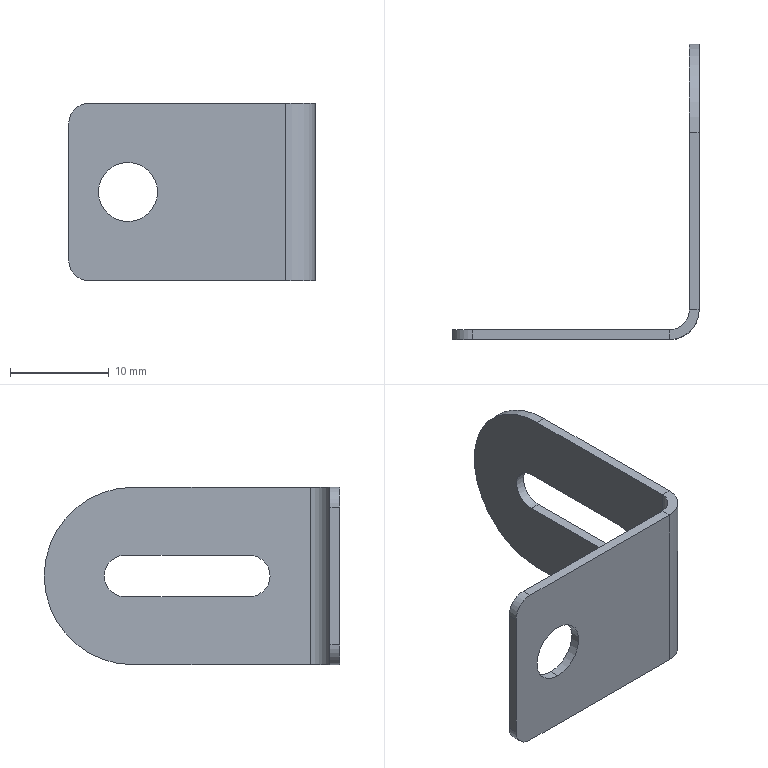Part | SolidWorks | features Fillet 2, ICE 2, EdgeFlange 1, FlatPattern 1, SMBaseFlange 1, SheetMetal 1 | 1 solid | 24 faces | box 25 x 30 x 18 mm | volume 820.964 mm3 | plane 13 | cylinder 11 | commonest cylinder face diameters 4 x3 4.2 x3 6 x3 18 x2
STEP:
#1=CARTESIAN_POINT('',(12.5,8.173,2.1));
#2=VERTEX_POINT('',#1);
#3=CARTESIAN_POINT('',(12.5,6.073,0.));
#4=VERTEX_POINT('',#3);
#5=CARTESIAN_POINT('',(12.5,8.173,0.));
#6=DIRECTION('',(1.,0.,0.));
#7=DIRECTION('',(0.,1.,0.));
#8=AXIS2_PLACEMENT_3D('',#5,#6,#7);
#9=CIRCLE('',#8,2.1);
#10=EDGE_CURVE('',#2,#4,#9,.T.);
#11=ORIENTED_EDGE('',*,*,#10,.T.);
#12=CARTESIAN_POINT('',(11.5,6.073,0.));
#13=VERTEX_POINT('',#12);
#14=CARTESIAN_POINT('',(21.5,6.073,0.));
#15=DIRECTION('',(-1.,0.,0.));
#16=VECTOR('',#15,1000.);
#17=LINE('',#14,#16);
#18=EDGE_CURVE('',#4,#13,#17,.T.);
#19=ORIENTED_EDGE('',*,*,#18,.T.);
#20=CARTESIAN_POINT('',(11.5,8.173,2.1));
#21=VERTEX_POINT('',#20);
#22=CARTESIAN_POINT('',(11.5,8.173,0.));
#23=DIRECTION('',(-1.,0.,0.));
#24=DIRECTION('',(0.,-1.,0.));
#25=AXIS2_PLACEMENT_3D('',#22,#23,#24);
#26=CIRCLE('',#25,2.1);
#27=EDGE_CURVE('',#13,#21,#26,.T.);
#28=ORIENTED_EDGE('',*,*,#27,.T.);
#29=CARTESIAN_POINT('',(21.5,8.173,2.1));
#30=DIRECTION('',(-1.,0.,0.));
#31=VECTOR('',#30,1000.);
#32=LINE('',#29,#31);
#33=EDGE_CURVE('',#2,#21,#32,.T.);
#34=ORIENTED_EDGE('',*,*,#33,.F.);
#35=EDGE_LOOP('',(#11,#19,#28,#34));
#36=FACE_OUTER_BOUND('',#35,.T.);
#37=CARTESIAN_POINT('',(21.5,8.173,0.));
#38=DIRECTION('',(-1.,0.,0.));
#39=DIRECTION('',(0.,-1.,0.));
#40=AXIS2_PLACEMENT_3D('',#37,#38,#39);
#41=CYLINDRICAL_SURFACE('',#40,2.1);
#42=ADVANCED_FACE('',(#36),#41,.F.);
#43=CARTESIAN_POINT('',(-6.5,-1.,-3.));
#44=VERTEX_POINT('',#43);
#45=CARTESIAN_POINT('',(-6.5,-1.,3.));
#46=VERTEX_POINT('',#45);
#47=CARTESIAN_POINT('',(-6.5,-1.,0.));
#48=DIRECTION('',(0.,1.,0.));
#49=DIRECTION('',(0.,0.,1.));
#50=AXIS2_PLACEMENT_3D('',#47,#48,#49);
#51=CIRCLE('',#50,3.);
#52=EDGE_CURVE('',#44,#46,#51,.T.);
#53=ORIENTED_EDGE('',*,*,#52,.F.);
#54=CARTESIAN_POINT('',(-6.5,0.,-3.));
#55=VERTEX_POINT('',#54);
#56=CARTESIAN_POINT('',(-6.5,-10.,-3.));
#57=DIRECTION('',(0.,1.,0.));
#58=VECTOR('',#57,1000.);
#59=LINE('',#56,#58);
#60=EDGE_CURVE('',#44,#55,#59,.T.);
#61=ORIENTED_EDGE('',*,*,#60,.T.);
#62=CARTESIAN_POINT('',(-6.5,0.,3.));
#63=VERTEX_POINT('',#62);
#64=CARTESIAN_POINT('',(-6.5,0.,0.));
#65=DIRECTION('',(0.,1.,0.));
#66=DIRECTION('',(0.,0.,1.));
#67=AXIS2_PLACEMENT_3D('',#64,#65,#66);
#68=CIRCLE('',#67,3.);
#69=EDGE_CURVE('',#55,#63,#68,.T.);
#70=ORIENTED_EDGE('',*,*,#69,.T.);
#71=CARTESIAN_POINT('',(-6.5,-10.,3.));
#72=DIRECTION('',(0.,1.,0.));
#73=VECTOR('',#72,1000.);
#74=LINE('',#71,#73);
#75=EDGE_CURVE('',#46,#63,#74,.T.);
#76=ORIENTED_EDGE('',*,*,#75,.F.);
#77=EDGE_LOOP('',(#53,#61,#70,#76));
#78=FACE_OUTER_BOUND('',#77,.T.);
#79=CARTESIAN_POINT('',(-6.5,-10.,0.));
#80=DIRECTION('',(0.,1.,0.));
#81=DIRECTION('',(0.,0.,1.));
#82=AXIS2_PLACEMENT_3D('',#79,#80,#81);
#83=CYLINDRICAL_SURFACE('',#82,3.);
#84=ADVANCED_FACE('',(#78),#83,.F.);
#85=CARTESIAN_POINT('',(9.5,-1.,-9.));
#86=VERTEX_POINT('',#85);
#87=CARTESIAN_POINT('',(-10.5,-1.,-9.));
#88=VERTEX_POINT('',#87);
#89=CARTESIAN_POINT('',(-12.5,-1.,-9.));
#90=DIRECTION('',(-1.,0.,0.));
#91=VECTOR('',#90,1000.);
#92=LINE('',#89,#91);
#93=EDGE_CURVE('',#86,#88,#92,.T.);
#94=ORIENTED_EDGE('',*,*,#93,.T.);
#95=CARTESIAN_POINT('',(-10.5,0.,-9.));
#96=VERTEX_POINT('',#95);
#97=CARTESIAN_POINT('',(-10.5,-1.,-9.));
#98=DIRECTION('',(0.,1.,0.));
#99=VECTOR('',#98,1000.);
#100=LINE('',#97,#99);
#101=EDGE_CURVE('',#88,#96,#100,.T.);
#102=ORIENTED_EDGE('',*,*,#101,.T.);
#103=CARTESIAN_POINT('',(9.5,0.,-9.));
#104=VERTEX_POINT('',#103);
#105=CARTESIAN_POINT('',(-12.5,0.,-9.));
#106=DIRECTION('',(-1.,0.,0.));
#107=VECTOR('',#106,1000.);
#108=LINE('',#105,#107);
#109=EDGE_CURVE('',#104,#96,#108,.T.);
#110=ORIENTED_EDGE('',*,*,#109,.F.);
#111=CARTESIAN_POINT('',(9.5,0.,-9.));
#112=DIRECTION('',(0.,-1.,0.));
#113=VECTOR('',#112,1000.);
#114=LINE('',#111,#113);
#115=EDGE_CURVE('',#104,#86,#114,.T.);
#116=ORIENTED_EDGE('',*,*,#115,.T.);
#117=EDGE_LOOP('',(#94,#102,#110,#116));
#118=FACE_OUTER_BOUND('',#117,.T.);
#119=CARTESIAN_POINT('',(-12.5,-1.,-9.));
#120=DIRECTION('',(0.,0.,-1.));
#121=DIRECTION('',(-1.,0.,0.));
#122=AXIS2_PLACEMENT_3D('',#119,#120,#121);
#123=PLANE('',#122);
#124=ADVANCED_FACE('',(#118),#123,.T.);
#125=CARTESIAN_POINT('',(-6.5,-1.,0.));
#126=DIRECTION('',(0.,1.,0.));
#127=DIRECTION('',(0.,0.,1.));
#128=AXIS2_PLACEMENT_3D('',#125,#126,#127);
#129=CIRCLE('',#128,3.);
#130=EDGE_CURVE('',#46,#44,#129,.T.);
#131=ORIENTED_EDGE('',*,*,#130,.T.);
#132=ORIENTED_EDGE('',*,*,#52,.T.);
#133=EDGE_LOOP('',(#131,#132));
#134=FACE_BOUND('',#133,.T.);
#135=CARTESIAN_POINT('',(-12.5,-1.,-7.));
#136=VERTEX_POINT('',#135);
#137=CARTESIAN_POINT('',(-12.5,-1.,7.));
#138=VERTEX_POINT('',#137);
#139=CARTESIAN_POINT('',(-12.5,-1.,-9.));
#140=DIRECTION('',(0.,0.,1.));
#141=VECTOR('',#140,1000.);
#142=LINE('',#139,#141);
#143=EDGE_CURVE('',#136,#138,#142,.T.);
#144=ORIENTED_EDGE('',*,*,#143,.F.);
#145=CARTESIAN_POINT('',(-10.5,-1.,-7.));
#146=DIRECTION('',(0.,-1.,0.));
#147=DIRECTION('',(0.,0.,1.));
#148=AXIS2_PLACEMENT_3D('',#145,#146,#147);
#149=CIRCLE('',#148,2.);
#150=EDGE_CURVE('',#136,#88,#149,.T.);
#151=ORIENTED_EDGE('',*,*,#150,.T.);
#152=ORIENTED_EDGE('',*,*,#93,.F.);
#153=CARTESIAN_POINT('',(9.5,-1.,9.));
#154=VERTEX_POINT('',#153);
#155=CARTESIAN_POINT('',(9.5,-1.,-9.));
#156=DIRECTION('',(0.,0.,1.));
#157=VECTOR('',#156,1000.);
#158=LINE('',#155,#157);
#159=EDGE_CURVE('',#86,#154,#158,.T.);
#160=ORIENTED_EDGE('',*,*,#159,.T.);
#161=CARTESIAN_POINT('',(-10.5,-1.,9.));
#162=VERTEX_POINT('',#161);
#163=CARTESIAN_POINT('',(-12.5,-1.,9.));
#164=DIRECTION('',(1.,0.,0.));
#165=VECTOR('',#164,1000.);
#166=LINE('',#163,#165);
#167=EDGE_CURVE('',#162,#154,#166,.T.);
#168=ORIENTED_EDGE('',*,*,#167,.F.);
#169=CARTESIAN_POINT('',(-10.5,-1.,7.));
#170=DIRECTION('',(0.,-1.,0.));
#171=DIRECTION('',(0.,0.,1.));
#172=AXIS2_PLACEMENT_3D('',#169,#170,#171);
#173=CIRCLE('',#172,2.);
#174=EDGE_CURVE('',#162,#138,#173,.T.);
#175=ORIENTED_EDGE('',*,*,#174,.T.);
#176=EDGE_LOOP('',(#144,#151,#152,#160,#168,#175));
#177=FACE_OUTER_BOUND('',#176,.T.);
#178=CARTESIAN_POINT('',(0.,-1.,0.));
#179=DIRECTION('',(0.,1.,0.));
#180=DIRECTION('',(0.,0.,1.));
#181=AXIS2_PLACEMENT_3D('',#178,#179,#180);
#182=PLANE('',#181);
#183=ADVANCED_FACE('',(#134,#177),#182,.F.);
#184=CARTESIAN_POINT('',(-6.5,0.,0.));
#185=DIRECTION('',(0.,1.,0.));
#186=DIRECTION('',(0.,0.,1.));
#187=AXIS2_PLACEMENT_3D('',#184,#185,#186);
#188=CIRCLE('',#187,3.);
#189=EDGE_CURVE('',#63,#55,#188,.T.);
#190=ORIENTED_EDGE('',*,*,#189,.F.);
#191=ORIENTED_EDGE('',*,*,#69,.F.);
#192=EDGE_LOOP('',(#190,#191));
#193=FACE_BOUND('',#192,.T.);
#194=ORIENTED_EDGE('',*,*,#109,.T.);
#195=CARTESIAN_POINT('',(-12.5,0.,-7.));
#196=VERTEX_POINT('',#195);
#197=CARTESIAN_POINT('',(-10.5,0.,-7.));
#198=DIRECTION('',(0.,1.,0.));
#199=DIRECTION('',(0.,0.,1.));
#200=AXIS2_PLACEMENT_3D('',#197,#198,#199);
#201=CIRCLE('',#200,2.);
#202=EDGE_CURVE('',#96,#196,#201,.T.);
#203=ORIENTED_EDGE('',*,*,#202,.T.);
#204=CARTESIAN_POINT('',(-12.5,0.,7.));
#205=VERTEX_POINT('',#204);
#206=CARTESIAN_POINT('',(-12.5,0.,-9.));
#207=DIRECTION('',(0.,0.,1.));
#208=VECTOR('',#207,1000.);
#209=LINE('',#206,#208);
#210=EDGE_CURVE('',#196,#205,#209,.T.);
#211=ORIENTED_EDGE('',*,*,#210,.T.);
#212=CARTESIAN_POINT('',(-10.5,0.,9.));
#213=VERTEX_POINT('',#212);
#214=CARTESIAN_POINT('',(-10.5,0.,7.));
#215=DIRECTION('',(0.,1.,0.));
#216=DIRECTION('',(0.,0.,1.));
#217=AXIS2_PLACEMENT_3D('',#214,#215,#216);
#218=CIRCLE('',#217,2.);
#219=EDGE_CURVE('',#205,#213,#218,.T.);
#220=ORIENTED_EDGE('',*,*,#219,.T.);
#221=CARTESIAN_POINT('',(9.5,0.,9.));
#222=VERTEX_POINT('',#221);
#223=CARTESIAN_POINT('',(-12.5,0.,9.));
#224=DIRECTION('',(1.,0.,0.));
#225=VECTOR('',#224,1000.);
#226=LINE('',#223,#225);
#227=EDGE_CURVE('',#213,#222,#226,.T.);
#228=ORIENTED_EDGE('',*,*,#227,.T.);
#229=CARTESIAN_POINT('',(9.5,0.,-9.));
#230=DIRECTION('',(0.,0.,1.));
#231=VECTOR('',#230,1000.);
#232=LINE('',#229,#231);
#233=EDGE_CURVE('',#104,#222,#232,.T.);
#234=ORIENTED_EDGE('',*,*,#233,.F.);
#235=EDGE_LOOP('',(#194,#203,#211,#220,#228,#234));
#236=FACE_OUTER_BOUND('',#235,.T.);
#237=CARTESIAN_POINT('',(0.,0.,0.));
#238=DIRECTION('',(0.,1.,0.));
#239=DIRECTION('',(0.,0.,1.));
#240=AXIS2_PLACEMENT_3D('',#237,#238,#239);
#241=PLANE('',#240);
#242=ADVANCED_FACE('',(#193,#236),#241,.T.);
#243=ORIENTED_EDGE('',*,*,#227,.F.);
#244=CARTESIAN_POINT('',(-10.5,-1.,9.));
#245=DIRECTION('',(0.,-1.,0.));
#246=VECTOR('',#245,1000.);
#247=LINE('',#244,#246);
#248=EDGE_CURVE('',#213,#162,#247,.T.);
#249=ORIENTED_EDGE('',*,*,#248,.T.);
#250=ORIENTED_EDGE('',*,*,#167,.T.);
#251=CARTESIAN_POINT('',(9.5,0.,9.));
#252=DIRECTION('',(0.,-1.,0.));
#253=VECTOR('',#252,1000.);
#254=LINE('',#251,#253);
#255=EDGE_CURVE('',#222,#154,#254,.T.);
#256=ORIENTED_EDGE('',*,*,#255,.F.);
#257=EDGE_LOOP('',(#243,#249,#250,#256));
#258=FACE_OUTER_BOUND('',#257,.T.);
#259=CARTESIAN_POINT('',(-12.5,-1.,9.));
#260=DIRECTION('',(0.,0.,1.));
#261=DIRECTION('',(1.,0.,0.));
#262=AXIS2_PLACEMENT_3D('',#259,#260,#261);
#263=PLANE('',#262);
#264=ADVANCED_FACE('',(#258),#263,.T.);
#265=ORIENTED_EDGE('',*,*,#210,.F.);
#266=CARTESIAN_POINT('',(-12.5,-1.,-7.));
#267=DIRECTION('',(0.,-1.,0.));
#268=VECTOR('',#267,1000.);
#269=LINE('',#266,#268);
#270=EDGE_CURVE('',#196,#136,#269,.T.);
#271=ORIENTED_EDGE('',*,*,#270,.T.);
#272=ORIENTED_EDGE('',*,*,#143,.T.);
#273=CARTESIAN_POINT('',(-12.5,-1.,7.));
#274=DIRECTION('',(0.,1.,0.));
#275=VECTOR('',#274,1000.);
#276=LINE('',#273,#275);
#277=EDGE_CURVE('',#138,#205,#276,.T.);
#278=ORIENTED_EDGE('',*,*,#277,.T.);
#279=EDGE_LOOP('',(#265,#271,#272,#278));
#280=FACE_OUTER_BOUND('',#279,.T.);
#281=CARTESIAN_POINT('',(-12.5,-1.,-9.));
#282=DIRECTION('',(-1.,0.,0.));
#283=DIRECTION('',(0.,0.,1.));
#284=AXIS2_PLACEMENT_3D('',#281,#282,#283);
#285=PLANE('',#284);
#286=ADVANCED_FACE('',(#280),#285,.T.);
#287=CARTESIAN_POINT('',(11.5,2.,9.));
#288=VERTEX_POINT('',#287);
#289=CARTESIAN_POINT('',(12.5,2.,9.));
#290=VERTEX_POINT('',#289);
#291=CARTESIAN_POINT('',(12.5,2.,9.));
#292=DIRECTION('',(1.,0.,0.));
#293=VECTOR('',#292,1000.);
#294=LINE('',#291,#293);
#295=EDGE_CURVE('',#288,#290,#294,.T.);
#296=ORIENTED_EDGE('',*,*,#295,.F.);
#297=CARTESIAN_POINT('',(9.5,2.,9.));
#298=DIRECTION('',(0.,0.,1.));
#299=DIRECTION('',(-1.,0.,0.));
#300=AXIS2_PLACEMENT_3D('',#297,#298,#299);
#301=CIRCLE('',#300,2.);
#302=EDGE_CURVE('',#222,#288,#301,.T.);
#303=ORIENTED_EDGE('',*,*,#302,.F.);
#304=ORIENTED_EDGE('',*,*,#255,.T.);
#305=CARTESIAN_POINT('',(9.5,2.,9.));
#306=DIRECTION('',(0.,0.,1.));
#307=DIRECTION('',(-1.,0.,0.));
#308=AXIS2_PLACEMENT_3D('',#305,#306,#307);
#309=CIRCLE('',#308,3.);
#310=EDGE_CURVE('',#154,#290,#309,.T.);
#311=ORIENTED_EDGE('',*,*,#310,.T.);
#312=EDGE_LOOP('',(#296,#303,#304,#311));
#313=FACE_OUTER_BOUND('',#312,.T.);
#314=CARTESIAN_POINT('',(9.5,2.,9.));
#315=DIRECTION('',(0.,0.,1.));
#316=DIRECTION('',(1.,0.,0.));
#317=AXIS2_PLACEMENT_3D('',#314,#315,#316);
#318=PLANE('',#317);
#319=ADVANCED_FACE('',(#313),#318,.T.);
#320=CARTESIAN_POINT('',(11.5,2.,-9.));
#321=VERTEX_POINT('',#320);
#322=CARTESIAN_POINT('',(9.5,2.,-9.));
#323=DIRECTION('',(0.,0.,-1.));
#324=DIRECTION('',(-1.,0.,0.));
#325=AXIS2_PLACEMENT_3D('',#322,#323,#324);
#326=CIRCLE('',#325,2.);
#327=EDGE_CURVE('',#321,#104,#326,.T.);
#328=ORIENTED_EDGE('',*,*,#327,.F.);
#329=CARTESIAN_POINT('',(12.5,2.,-9.));
#330=VERTEX_POINT('',#329);
#331=CARTESIAN_POINT('',(11.5,2.,-9.));
#332=DIRECTION('',(1.,0.,0.));
#333=VECTOR('',#332,1000.);
#334=LINE('',#331,#333);
#335=EDGE_CURVE('',#321,#330,#334,.T.);
#336=ORIENTED_EDGE('',*,*,#335,.T.);
#337=CARTESIAN_POINT('',(9.5,2.,-9.));
#338=DIRECTION('',(0.,0.,-1.));
#339=DIRECTION('',(-1.,0.,0.));
#340=AXIS2_PLACEMENT_3D('',#337,#338,#339);
#341=CIRCLE('',#340,3.);
#342=EDGE_CURVE('',#330,#86,#341,.T.);
#343=ORIENTED_EDGE('',*,*,#342,.T.);
#344=ORIENTED_EDGE('',*,*,#115,.F.);
#345=EDGE_LOOP('',(#328,#336,#343,#344));
#346=FACE_OUTER_BOUND('',#345,.T.);
#347=CARTESIAN_POINT('',(9.5,2.,-9.));
#348=DIRECTION('',(0.,0.,1.));
#349=DIRECTION('',(1.,0.,0.));
#350=AXIS2_PLACEMENT_3D('',#347,#348,#349);
#351=PLANE('',#350);
#352=ADVANCED_FACE('',(#346),#351,.F.);
#353=ORIENTED_EDGE('',*,*,#159,.F.);
#354=ORIENTED_EDGE('',*,*,#342,.F.);
#355=CARTESIAN_POINT('',(12.5,2.,0.));
#356=DIRECTION('',(0.,0.,-1.));
#357=VECTOR('',#356,1000.);
#358=LINE('',#355,#357);
#359=EDGE_CURVE('',#290,#330,#358,.T.);
#360=ORIENTED_EDGE('',*,*,#359,.F.);
#361=ORIENTED_EDGE('',*,*,#310,.F.);
#362=EDGE_LOOP('',(#353,#354,#360,#361));
#363=FACE_OUTER_BOUND('',#362,.T.);
#364=CARTESIAN_POINT('',(9.5,2.,-9.));
#365=DIRECTION('',(0.,0.,-1.));
#366=DIRECTION('',(1.,0.,0.));
#367=AXIS2_PLACEMENT_3D('',#364,#365,#366);
#368=CYLINDRICAL_SURFACE('',#367,3.);
#369=ADVANCED_FACE('',(#363),#368,.T.);
#370=ORIENTED_EDGE('',*,*,#233,.T.);
#371=ORIENTED_EDGE('',*,*,#302,.T.);
#372=CARTESIAN_POINT('',(11.5,2.,9.));
#373=DIRECTION('',(0.,0.,-1.));
#374=VECTOR('',#373,1000.);
#375=LINE('',#372,#374);
#376=EDGE_CURVE('',#288,#321,#375,.T.);
#377=ORIENTED_EDGE('',*,*,#376,.T.);
#378=ORIENTED_EDGE('',*,*,#327,.T.);
#379=EDGE_LOOP('',(#370,#371,#377,#378));
#380=FACE_OUTER_BOUND('',#379,.T.);
#381=CARTESIAN_POINT('',(9.5,2.,-9.));
#382=DIRECTION('',(0.,0.,-1.));
#383=DIRECTION('',(1.,0.,0.));
#384=AXIS2_PLACEMENT_3D('',#381,#382,#383);
#385=CYLINDRICAL_SURFACE('',#384,2.);
#386=ADVANCED_FACE('',(#380),#385,.F.);
#387=CARTESIAN_POINT('',(11.5,20.,-9.));
#388=VERTEX_POINT('',#387);
#389=CARTESIAN_POINT('',(11.5,0.,-9.));
#390=DIRECTION('',(0.,-1.,0.));
#391=VECTOR('',#390,1000.);
#392=LINE('',#389,#391);
#393=EDGE_CURVE('',#388,#321,#392,.T.);
#394=ORIENTED_EDGE('',*,*,#393,.F.);
#395=CARTESIAN_POINT('',(12.5,20.,-9.));
#396=VERTEX_POINT('',#395);
#397=CARTESIAN_POINT('',(12.5,20.,-9.));
#398=DIRECTION('',(1.,0.,0.));
#399=VECTOR('',#398,1000.);
#400=LINE('',#397,#399);
#401=EDGE_CURVE('',#388,#396,#400,.T.);
#402=ORIENTED_EDGE('',*,*,#401,.T.);
#403=CARTESIAN_POINT('',(12.5,0.,-9.));
#404=DIRECTION('',(0.,-1.,0.));
#405=VECTOR('',#404,1000.);
#406=LINE('',#403,#405);
#407=EDGE_CURVE('',#396,#330,#406,.T.);
#408=ORIENTED_EDGE('',*,*,#407,.T.);
#409=ORIENTED_EDGE('',*,*,#335,.F.);
#410=EDGE_LOOP('',(#394,#402,#408,#409));
#411=FACE_OUTER_BOUND('',#410,.T.);
#412=CARTESIAN_POINT('',(12.5,0.,-9.));
#413=DIRECTION('',(0.,0.,-1.));
#414=DIRECTION('',(-1.,0.,0.));
#415=AXIS2_PLACEMENT_3D('',#412,#413,#414);
#416=PLANE('',#415);
#417=ADVANCED_FACE('',(#411),#416,.T.);
#418=CARTESIAN_POINT('',(12.5,20.,9.));
#419=VERTEX_POINT('',#418);
#420=CARTESIAN_POINT('',(12.5,29.,9.));
#421=DIRECTION('',(0.,1.,0.));
#422=VECTOR('',#421,1000.);
#423=LINE('',#420,#422);
#424=EDGE_CURVE('',#290,#419,#423,.T.);
#425=ORIENTED_EDGE('',*,*,#424,.T.);
#426=CARTESIAN_POINT('',(11.5,20.,9.));
#427=VERTEX_POINT('',#426);
#428=CARTESIAN_POINT('',(12.5,20.,9.));
#429=DIRECTION('',(-1.,0.,0.));
#430=VECTOR('',#429,1000.);
#431=LINE('',#428,#430);
#432=EDGE_CURVE('',#419,#427,#431,.T.);
#433=ORIENTED_EDGE('',*,*,#432,.T.);
#434=CARTESIAN_POINT('',(11.5,0.,9.));
#435=DIRECTION('',(0.,1.,0.));
#436=VECTOR('',#435,1000.);
#437=LINE('',#434,#436);
#438=EDGE_CURVE('',#288,#427,#437,.T.);
#439=ORIENTED_EDGE('',*,*,#438,.F.);
#440=ORIENTED_EDGE('',*,*,#295,.T.);
#441=EDGE_LOOP('',(#425,#433,#439,#440));
#442=FACE_OUTER_BOUND('',#441,.T.);
#443=CARTESIAN_POINT('',(12.5,29.,9.));
#444=DIRECTION('',(0.,0.,1.));
#445=DIRECTION('',(1.,0.,0.));
#446=AXIS2_PLACEMENT_3D('',#443,#444,#445);
#447=PLANE('',#446);
#448=ADVANCED_FACE('',(#442),#447,.T.);
#449=CARTESIAN_POINT('',(12.5,20.819,-2.1));
#450=VERTEX_POINT('',#449);
#451=CARTESIAN_POINT('',(12.5,20.819,2.1));
#452=VERTEX_POINT('',#451);
#453=CARTESIAN_POINT('',(12.5,20.819,0.));
#454=DIRECTION('',(1.,0.,0.));
#455=DIRECTION('',(0.,1.,0.));
#456=AXIS2_PLACEMENT_3D('',#453,#454,#455);
#457=CIRCLE('',#456,2.1);
#458=EDGE_CURVE('',#450,#452,#457,.T.);
#459=ORIENTED_EDGE('',*,*,#458,.F.);
#460=CARTESIAN_POINT('',(12.5,8.173,-2.1));
#461=VERTEX_POINT('',#460);
#462=CARTESIAN_POINT('',(12.5,0.,-2.1));
#463=DIRECTION('',(0.,1.,0.));
#464=VECTOR('',#463,1000.);
#465=LINE('',#462,#464);
#466=EDGE_CURVE('',#461,#450,#465,.T.);
#467=ORIENTED_EDGE('',*,*,#466,.F.);
#468=CARTESIAN_POINT('',(12.5,8.173,0.));
#469=DIRECTION('',(1.,0.,0.));
#470=DIRECTION('',(0.,1.,0.));
#471=AXIS2_PLACEMENT_3D('',#468,#469,#470);
#472=CIRCLE('',#471,2.1);
#473=EDGE_CURVE('',#4,#461,#472,.T.);
#474=ORIENTED_EDGE('',*,*,#473,.F.);
#475=ORIENTED_EDGE('',*,*,#10,.F.);
#476=CARTESIAN_POINT('',(12.5,0.,2.1));
#477=DIRECTION('',(0.,-1.,0.));
#478=VECTOR('',#477,1000.);
#479=LINE('',#476,#478);
#480=EDGE_CURVE('',#452,#2,#479,.T.);
#481=ORIENTED_EDGE('',*,*,#480,.F.);
#482=EDGE_LOOP('',(#459,#467,#474,#475,#481));
#483=FACE_BOUND('',#482,.T.);
#484=ORIENTED_EDGE('',*,*,#407,.F.);
#485=CARTESIAN_POINT('',(12.5,29.,0.));
#486=VERTEX_POINT('',#485);
#487=CARTESIAN_POINT('',(12.5,20.,0.));
#488=DIRECTION('',(1.,0.,0.));
#489=DIRECTION('',(0.,1.,0.));
#490=AXIS2_PLACEMENT_3D('',#487,#488,#489);
#491=CIRCLE('',#490,9.);
#492=EDGE_CURVE('',#396,#486,#491,.T.);
#493=ORIENTED_EDGE('',*,*,#492,.T.);
#494=CARTESIAN_POINT('',(12.5,20.,0.));
#495=DIRECTION('',(1.,0.,0.));
#496=DIRECTION('',(0.,1.,0.));
#497=AXIS2_PLACEMENT_3D('',#494,#495,#496);
#498=CIRCLE('',#497,9.);
#499=EDGE_CURVE('',#486,#419,#498,.T.);
#500=ORIENTED_EDGE('',*,*,#499,.T.);
#501=ORIENTED_EDGE('',*,*,#424,.F.);
#502=ORIENTED_EDGE('',*,*,#359,.T.);
#503=EDGE_LOOP('',(#484,#493,#500,#501,#502));
#504=FACE_OUTER_BOUND('',#503,.T.);
#505=CARTESIAN_POINT('',(12.5,0.,0.));
#506=DIRECTION('',(1.,0.,0.));
#507=DIRECTION('',(0.,1.,0.));
#508=AXIS2_PLACEMENT_3D('',#505,#506,#507);
#509=PLANE('',#508);
#510=ADVANCED_FACE('',(#483,#504),#509,.T.);
#511=CARTESIAN_POINT('',(11.5,20.819,-2.1));
#512=VERTEX_POINT('',#511);
#513=CARTESIAN_POINT('',(11.5,8.173,-2.1));
#514=VERTEX_POINT('',#513);
#515=CARTESIAN_POINT('',(11.5,20.819,-2.1));
#516=DIRECTION('',(0.,-1.,0.));
#517=VECTOR('',#516,1000.);
#518=LINE('',#515,#517);
#519=EDGE_CURVE('',#512,#514,#518,.T.);
#520=ORIENTED_EDGE('',*,*,#519,.F.);
#521=CARTESIAN_POINT('',(11.5,20.819,2.1));
#522=VERTEX_POINT('',#521);
#523=CARTESIAN_POINT('',(11.5,20.819,0.));
#524=DIRECTION('',(-1.,0.,0.));
#525=DIRECTION('',(0.,-1.,0.));
#526=AXIS2_PLACEMENT_3D('',#523,#524,#525);
#527=CIRCLE('',#526,2.1);
#528=EDGE_CURVE('',#522,#512,#527,.T.);
#529=ORIENTED_EDGE('',*,*,#528,.F.);
#530=CARTESIAN_POINT('',(11.5,20.819,2.1));
#531=DIRECTION('',(0.,1.,0.));
#532=VECTOR('',#531,1000.);
#533=LINE('',#530,#532);
#534=EDGE_CURVE('',#21,#522,#533,.T.);
#535=ORIENTED_EDGE('',*,*,#534,.F.);
#536=ORIENTED_EDGE('',*,*,#27,.F.);
#537=CARTESIAN_POINT('',(11.5,8.173,0.));
#538=DIRECTION('',(-1.,0.,0.));
#539=DIRECTION('',(0.,-1.,0.));
#540=AXIS2_PLACEMENT_3D('',#537,#538,#539);
#541=CIRCLE('',#540,2.1);
#542=EDGE_CURVE('',#514,#13,#541,.T.);
#543=ORIENTED_EDGE('',*,*,#542,.F.);
#544=EDGE_LOOP('',(#520,#529,#535,#536,#543));
#545=FACE_BOUND('',#544,.T.);
#546=CARTESIAN_POINT('',(11.5,29.,0.));
#547=VERTEX_POINT('',#546);
#548=CARTESIAN_POINT('',(11.5,20.,0.));
#549=DIRECTION('',(-1.,0.,0.));
#550=DIRECTION('',(0.,1.,0.));
#551=AXIS2_PLACEMENT_3D('',#548,#549,#550);
#552=CIRCLE('',#551,9.);
#553=EDGE_CURVE('',#427,#547,#552,.T.);
#554=ORIENTED_EDGE('',*,*,#553,.T.);
#555=CARTESIAN_POINT('',(11.5,20.,0.));
#556=DIRECTION('',(-1.,0.,0.));
#557=DIRECTION('',(0.,1.,0.));
#558=AXIS2_PLACEMENT_3D('',#555,#556,#557);
#559=CIRCLE('',#558,9.);
#560=EDGE_CURVE('',#547,#388,#559,.T.);
#561=ORIENTED_EDGE('',*,*,#560,.T.);
#562=ORIENTED_EDGE('',*,*,#393,.T.);
#563=ORIENTED_EDGE('',*,*,#376,.F.);
#564=ORIENTED_EDGE('',*,*,#438,.T.);
#565=EDGE_LOOP('',(#554,#561,#562,#563,#564));
#566=FACE_OUTER_BOUND('',#565,.T.);
#567=CARTESIAN_POINT('',(11.5,0.,0.));
#568=DIRECTION('',(1.,0.,0.));
#569=DIRECTION('',(0.,1.,0.));
#570=AXIS2_PLACEMENT_3D('',#567,#568,#569);
#571=PLANE('',#570);
#572=ADVANCED_FACE('',(#545,#566),#571,.F.);
#573=ORIENTED_EDGE('',*,*,#60,.F.);
#574=ORIENTED_EDGE('',*,*,#130,.F.);
#575=ORIENTED_EDGE('',*,*,#75,.T.);
#576=ORIENTED_EDGE('',*,*,#189,.T.);
#577=EDGE_LOOP('',(#573,#574,#575,#576));
#578=FACE_OUTER_BOUND('',#577,.T.);
#579=CARTESIAN_POINT('',(-6.5,-10.,0.));
#580=DIRECTION('',(0.,1.,0.));
#581=DIRECTION('',(0.,0.,1.));
#582=AXIS2_PLACEMENT_3D('',#579,#580,#581);
#583=CYLINDRICAL_SURFACE('',#582,3.);
#584=ADVANCED_FACE('',(#578),#583,.F.);
#585=ORIENTED_EDGE('',*,*,#432,.F.);
#586=ORIENTED_EDGE('',*,*,#499,.F.);
#587=CARTESIAN_POINT('',(12.5,29.,0.));
#588=DIRECTION('',(1.,0.,0.));
#589=VECTOR('',#588,1000.);
#590=LINE('',#587,#589);
#591=EDGE_CURVE('',#547,#486,#590,.T.);
#592=ORIENTED_EDGE('',*,*,#591,.F.);
#593=ORIENTED_EDGE('',*,*,#553,.F.);
#594=EDGE_LOOP('',(#585,#586,#592,#593));
#595=FACE_OUTER_BOUND('',#594,.T.);
#596=CARTESIAN_POINT('',(12.5,20.,0.));
#597=DIRECTION('',(-1.,0.,0.));
#598=DIRECTION('',(0.,-1.,0.));
#599=AXIS2_PLACEMENT_3D('',#596,#597,#598);
#600=CYLINDRICAL_SURFACE('',#599,9.);
#601=ADVANCED_FACE('',(#595),#600,.T.);
#602=ORIENTED_EDGE('',*,*,#492,.F.);
#603=ORIENTED_EDGE('',*,*,#401,.F.);
#604=ORIENTED_EDGE('',*,*,#560,.F.);
#605=ORIENTED_EDGE('',*,*,#591,.T.);
#606=EDGE_LOOP('',(#602,#603,#604,#605));
#607=FACE_OUTER_BOUND('',#606,.T.);
#608=CARTESIAN_POINT('',(12.5,20.,0.));
#609=DIRECTION('',(-1.,0.,0.));
#610=DIRECTION('',(0.,-1.,0.));
#611=AXIS2_PLACEMENT_3D('',#608,#609,#610);
#612=CYLINDRICAL_SURFACE('',#611,9.);
#613=ADVANCED_FACE('',(#607),#612,.T.);
#614=ORIENTED_EDGE('',*,*,#458,.T.);
#615=CARTESIAN_POINT('',(21.5,20.819,2.1));
#616=DIRECTION('',(-1.,0.,0.));
#617=VECTOR('',#616,1000.);
#618=LINE('',#615,#617);
#619=EDGE_CURVE('',#452,#522,#618,.T.);
#620=ORIENTED_EDGE('',*,*,#619,.T.);
#621=ORIENTED_EDGE('',*,*,#528,.T.);
#622=CARTESIAN_POINT('',(21.5,20.819,-2.1));
#623=DIRECTION('',(-1.,0.,0.));
#624=VECTOR('',#623,1000.);
#625=LINE('',#622,#624);
#626=EDGE_CURVE('',#450,#512,#625,.T.);
#627=ORIENTED_EDGE('',*,*,#626,.F.);
#628=EDGE_LOOP('',(#614,#620,#621,#627));
#629=FACE_OUTER_BOUND('',#628,.T.);
#630=CARTESIAN_POINT('',(21.5,20.819,0.));
#631=DIRECTION('',(-1.,0.,0.));
#632=DIRECTION('',(0.,-1.,0.));
#633=AXIS2_PLACEMENT_3D('',#630,#631,#632);
#634=CYLINDRICAL_SURFACE('',#633,2.1);
#635=ADVANCED_FACE('',(#629),#634,.F.);
#636=ORIENTED_EDGE('',*,*,#480,.T.);
#637=ORIENTED_EDGE('',*,*,#33,.T.);
#638=ORIENTED_EDGE('',*,*,#534,.T.);
#639=ORIENTED_EDGE('',*,*,#619,.F.);
#640=EDGE_LOOP('',(#636,#637,#638,#639));
#641=FACE_OUTER_BOUND('',#640,.T.);
#642=CARTESIAN_POINT('',(21.5,20.819,2.1));
#643=DIRECTION('',(0.,0.,1.));
#644=DIRECTION('',(1.,0.,0.));
#645=AXIS2_PLACEMENT_3D('',#642,#643,#644);
#646=PLANE('',#645);
#647=ADVANCED_FACE('',(#641),#646,.F.);
#648=ORIENTED_EDGE('',*,*,#18,.F.);
#649=ORIENTED_EDGE('',*,*,#473,.T.);
#650=CARTESIAN_POINT('',(21.5,8.173,-2.1));
#651=DIRECTION('',(-1.,0.,0.));
#652=VECTOR('',#651,1000.);
#653=LINE('',#650,#652);
#654=EDGE_CURVE('',#461,#514,#653,.T.);
#655=ORIENTED_EDGE('',*,*,#654,.T.);
#656=ORIENTED_EDGE('',*,*,#542,.T.);
#657=EDGE_LOOP('',(#648,#649,#655,#656));
#658=FACE_OUTER_BOUND('',#657,.T.);
#659=CARTESIAN_POINT('',(21.5,8.173,0.));
#660=DIRECTION('',(-1.,0.,0.));
#661=DIRECTION('',(0.,-1.,0.));
#662=AXIS2_PLACEMENT_3D('',#659,#660,#661);
#663=CYLINDRICAL_SURFACE('',#662,2.1);
#664=ADVANCED_FACE('',(#658),#663,.F.);
#665=ORIENTED_EDGE('',*,*,#466,.T.);
#666=ORIENTED_EDGE('',*,*,#626,.T.);
#667=ORIENTED_EDGE('',*,*,#519,.T.);
#668=ORIENTED_EDGE('',*,*,#654,.F.);
#669=EDGE_LOOP('',(#665,#666,#667,#668));
#670=FACE_OUTER_BOUND('',#669,.T.);
#671=CARTESIAN_POINT('',(21.5,20.819,-2.1));
#672=DIRECTION('',(0.,0.,-1.));
#673=DIRECTION('',(-1.,0.,0.));
#674=AXIS2_PLACEMENT_3D('',#671,#672,#673);
#675=PLANE('',#674);
#676=ADVANCED_FACE('',(#670),#675,.F.);
#677=ORIENTED_EDGE('',*,*,#150,.F.);
#678=ORIENTED_EDGE('',*,*,#270,.F.);
#679=ORIENTED_EDGE('',*,*,#202,.F.);
#680=ORIENTED_EDGE('',*,*,#101,.F.);
#681=EDGE_LOOP('',(#677,#678,#679,#680));
#682=FACE_OUTER_BOUND('',#681,.T.);
#683=CARTESIAN_POINT('',(-10.5,-1.,-7.));
#684=DIRECTION('',(0.,1.,0.));
#685=DIRECTION('',(0.,0.,1.));
#686=AXIS2_PLACEMENT_3D('',#683,#684,#685);
#687=CYLINDRICAL_SURFACE('',#686,2.);
#688=ADVANCED_FACE('',(#682),#687,.T.);
#689=ORIENTED_EDGE('',*,*,#174,.F.);
#690=ORIENTED_EDGE('',*,*,#248,.F.);
#691=ORIENTED_EDGE('',*,*,#219,.F.);
#692=ORIENTED_EDGE('',*,*,#277,.F.);
#693=EDGE_LOOP('',(#689,#690,#691,#692));
#694=FACE_OUTER_BOUND('',#693,.T.);
#695=CARTESIAN_POINT('',(-10.5,-1.,7.));
#696=DIRECTION('',(0.,1.,0.));
#697=DIRECTION('',(0.,0.,1.));
#698=AXIS2_PLACEMENT_3D('',#695,#696,#697);
#699=CYLINDRICAL_SURFACE('',#698,2.);
#700=ADVANCED_FACE('',(#694),#699,.T.);
#701=CLOSED_SHELL('',(#42,#84,#124,#183,#242,#264,#286,#319,#352,#369,#386,#417,#448,#510,#572,#584,#601,#613,#635,#647,#664,#676,#688,#700));
#702=MANIFOLD_SOLID_BREP('',#701);
#703=CARTESIAN_POINT('',(0.,0.,0.));
#704=DIRECTION('',(0.,0.,1.));
#705=DIRECTION('',(1.,0.,0.));
#706=AXIS2_PLACEMENT_3D('',#703,#704,#705);
#707=(LENGTH_UNIT()NAMED_UNIT(*)SI_UNIT(.MILLI.,.METRE.));
#708=UNCERTAINTY_MEASURE_WITH_UNIT(LENGTH_MEASURE(0.00001),#707,'','');
#709=(NAMED_UNIT(*)PLANE_ANGLE_UNIT()SI_UNIT($,.RADIAN.));
#710=(NAMED_UNIT(*)SI_UNIT($,.STERADIAN.)SOLID_ANGLE_UNIT());
#711=(GEOMETRIC_REPRESENTATION_CONTEXT(3)GLOBAL_UNCERTAINTY_ASSIGNED_CONTEXT((#708))GLOBAL_UNIT_ASSIGNED_CONTEXT((#707,#709,#710))REPRESENTATION_CONTEXT('',''));
#712=ADVANCED_BREP_SHAPE_REPRESENTATION('',(#702,#706),#711);